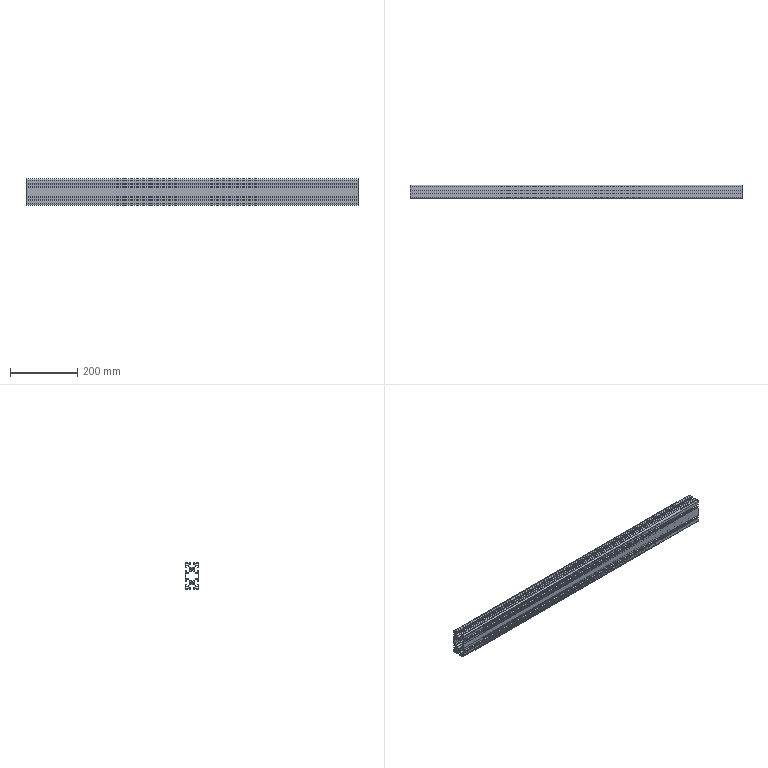Part | STEP file | Profile MK-8-4080H-L-05 4080H standard 990mm | 1 solid | 286 faces | box 990 x 40 x 80 mm | volume 803657 mm3 | cylinder 144 | plane 142 | commonest cylinder face diameters 0.6 x44 2 x44 4 x28 0.4 x14 6 x4 6.8 x4